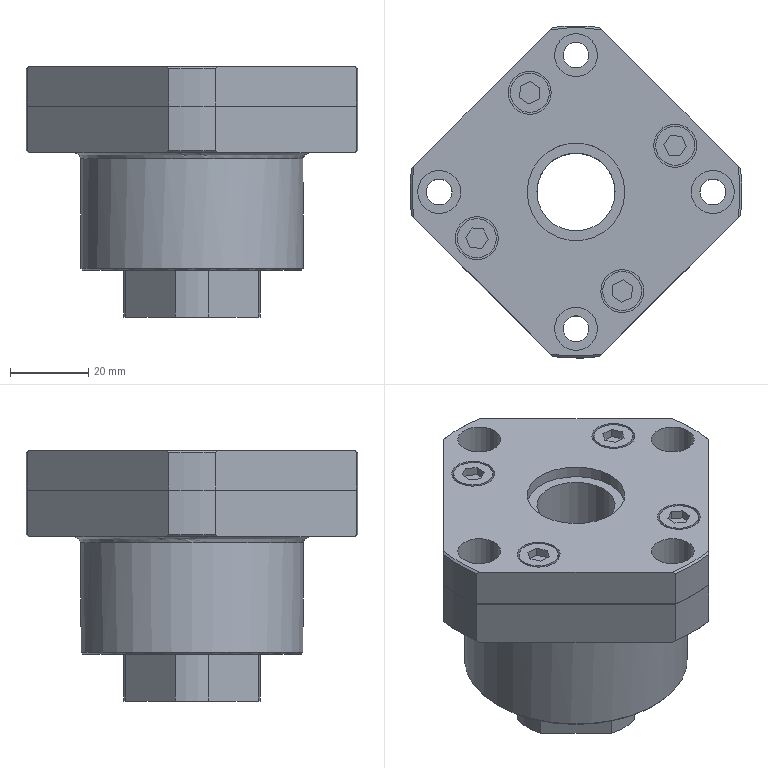Part | NX | 1 solid | 119 faces | box 85 x 85 x 64 mm | volume 157401 mm3 | plane 68 | cylinder 40 | cone 10 | spline 1 | commonest cylinder face diameters 11 x8 85 x8 6.6 x4 10 x4 35 x4 84.96 x4